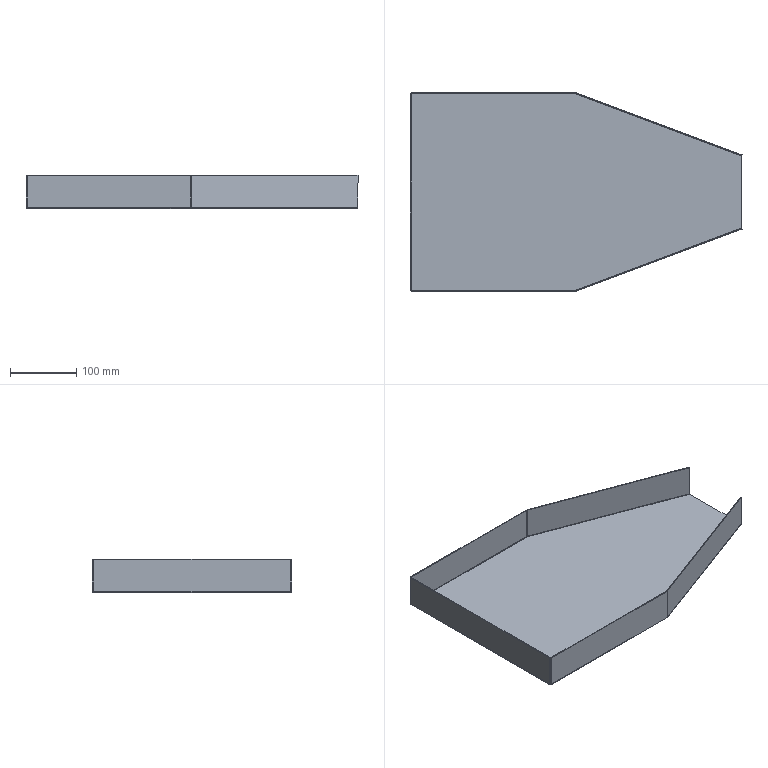Part | SolidWorks | features EdgeFlange 1, FlatPattern 1, SMBaseFlange 1, SheetMetal 1 | 1 solid | 54 faces | box 500 x 300 x 50 mm | volume 284706 mm3 | plane 36 | cylinder 10 | spline 8 | commonest cylinder face diameters 1 x5 4 x5